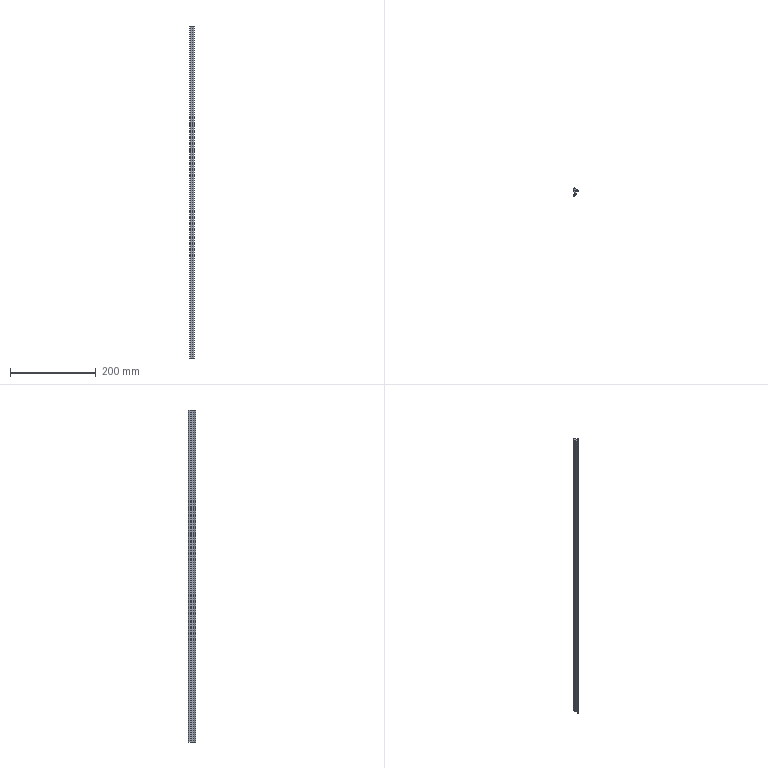Part | SolidWorks | features BaseBody 1, MoveFace 1 | 1 solid | 20 faces | box 10.8 x 17.5 x 774 mm | volume 60992 mm3 | cylinder 11 | plane 9 | commonest cylinder face diameters 1.6 x2 14 x2 0.4 x1 0.6 x1 0.8 x1 2.6 x1
STEP:
#1=CARTESIAN_POINT('',(-3.236,-11.055,674.));
#2=VERTEX_POINT('',#1);
#3=CARTESIAN_POINT('',(-4.3,-10.3,674.));
#4=VERTEX_POINT('',#3);
#5=CARTESIAN_POINT('',(-3.5,-10.3,674.));
#6=DIRECTION('',(0.,0.,-1.));
#7=DIRECTION('',(1.,0.,0.));
#8=AXIS2_PLACEMENT_3D('',#5,#6,#7);
#9=CIRCLE('',#8,0.8);
#10=EDGE_CURVE('',#2,#4,#9,.T.);
#11=ORIENTED_EDGE('',*,*,#10,.T.);
#12=CARTESIAN_POINT('',(-4.3,-10.3,-100.));
#13=VERTEX_POINT('',#12);
#14=CARTESIAN_POINT('',(-4.3,-10.3,-100.));
#15=DIRECTION('',(0.,0.,-1.));
#16=VECTOR('',#15,1000.);
#17=LINE('',#14,#16);
#18=EDGE_CURVE('',#4,#13,#17,.T.);
#19=ORIENTED_EDGE('',*,*,#18,.T.);
#20=CARTESIAN_POINT('',(-3.236,-11.055,-100.));
#21=VERTEX_POINT('',#20);
#22=CARTESIAN_POINT('',(-3.5,-10.3,-100.));
#23=DIRECTION('',(0.,0.,1.));
#24=DIRECTION('',(-1.,0.,0.));
#25=AXIS2_PLACEMENT_3D('',#22,#23,#24);
#26=CIRCLE('',#25,0.8);
#27=EDGE_CURVE('',#13,#21,#26,.T.);
#28=ORIENTED_EDGE('',*,*,#27,.T.);
#29=CARTESIAN_POINT('',(-3.236,-11.055,-100.));
#30=DIRECTION('',(0.,0.,-1.));
#31=VECTOR('',#30,1000.);
#32=LINE('',#29,#31);
#33=EDGE_CURVE('',#2,#21,#32,.T.);
#34=ORIENTED_EDGE('',*,*,#33,.F.);
#35=EDGE_LOOP('',(#11,#19,#28,#34));
#36=FACE_OUTER_BOUND('',#35,.T.);
#37=CARTESIAN_POINT('',(-3.5,-10.3,-100.));
#38=DIRECTION('',(0.,0.,-1.));
#39=DIRECTION('',(-1.,0.,0.));
#40=AXIS2_PLACEMENT_3D('',#37,#38,#39);
#41=CYLINDRICAL_SURFACE('',#40,0.8);
#42=ADVANCED_FACE('',(#36),#41,.T.);
#43=CARTESIAN_POINT('',(1.184,-6.397,-100.));
#44=VERTEX_POINT('',#43);
#45=CARTESIAN_POINT('',(-5.702,-4.29,-100.));
#46=DIRECTION('',(0.,0.,1.));
#47=DIRECTION('',(-1.,0.,0.));
#48=AXIS2_PLACEMENT_3D('',#45,#46,#47);
#49=CIRCLE('',#48,7.201);
#50=EDGE_CURVE('',#21,#44,#49,.T.);
#51=ORIENTED_EDGE('',*,*,#50,.T.);
#52=CARTESIAN_POINT('',(1.184,-6.397,674.));
#53=VERTEX_POINT('',#52);
#54=CARTESIAN_POINT('',(1.184,-6.397,-100.));
#55=DIRECTION('',(0.,0.,1.));
#56=VECTOR('',#55,1000.);
#57=LINE('',#54,#56);
#58=EDGE_CURVE('',#44,#53,#57,.T.);
#59=ORIENTED_EDGE('',*,*,#58,.T.);
#60=CARTESIAN_POINT('',(-5.702,-4.29,674.));
#61=DIRECTION('',(0.,0.,-1.));
#62=DIRECTION('',(1.,0.,0.));
#63=AXIS2_PLACEMENT_3D('',#60,#61,#62);
#64=CIRCLE('',#63,7.201);
#65=EDGE_CURVE('',#53,#2,#64,.T.);
#66=ORIENTED_EDGE('',*,*,#65,.T.);
#67=ORIENTED_EDGE('',*,*,#33,.T.);
#68=EDGE_LOOP('',(#51,#59,#66,#67));
#69=FACE_OUTER_BOUND('',#68,.T.);
#70=CARTESIAN_POINT('',(-5.702,-4.29,-100.));
#71=DIRECTION('',(0.,0.,-1.));
#72=DIRECTION('',(-1.,0.,0.));
#73=AXIS2_PLACEMENT_3D('',#70,#71,#72);
#74=CYLINDRICAL_SURFACE('',#73,7.201);
#75=ADVANCED_FACE('',(#69),#74,.T.);
#76=CARTESIAN_POINT('',(0.9,-6.,-100.));
#77=VERTEX_POINT('',#76);
#78=CARTESIAN_POINT('',(0.9,-6.3,-100.));
#79=DIRECTION('',(0.,0.,1.));
#80=DIRECTION('',(-1.,0.,0.));
#81=AXIS2_PLACEMENT_3D('',#78,#79,#80);
#82=CIRCLE('',#81,0.3);
#83=EDGE_CURVE('',#44,#77,#82,.T.);
#84=ORIENTED_EDGE('',*,*,#83,.T.);
#85=CARTESIAN_POINT('',(0.9,-6.,674.));
#86=VERTEX_POINT('',#85);
#87=CARTESIAN_POINT('',(0.9,-6.,-100.));
#88=DIRECTION('',(0.,0.,1.));
#89=VECTOR('',#88,1000.);
#90=LINE('',#87,#89);
#91=EDGE_CURVE('',#77,#86,#90,.T.);
#92=ORIENTED_EDGE('',*,*,#91,.T.);
#93=CARTESIAN_POINT('',(0.9,-6.3,674.));
#94=DIRECTION('',(0.,0.,-1.));
#95=DIRECTION('',(1.,0.,0.));
#96=AXIS2_PLACEMENT_3D('',#93,#94,#95);
#97=CIRCLE('',#96,0.3);
#98=EDGE_CURVE('',#86,#53,#97,.T.);
#99=ORIENTED_EDGE('',*,*,#98,.T.);
#100=ORIENTED_EDGE('',*,*,#58,.F.);
#101=EDGE_LOOP('',(#84,#92,#99,#100));
#102=FACE_OUTER_BOUND('',#101,.T.);
#103=CARTESIAN_POINT('',(0.9,-6.3,-100.));
#104=DIRECTION('',(0.,0.,-1.));
#105=DIRECTION('',(-1.,0.,0.));
#106=AXIS2_PLACEMENT_3D('',#103,#104,#105);
#107=CYLINDRICAL_SURFACE('',#106,0.3);
#108=ADVANCED_FACE('',(#102),#107,.T.);
#109=CARTESIAN_POINT('',(-2.5,-0.5,-100.));
#110=VERTEX_POINT('',#109);
#111=CARTESIAN_POINT('',(-2.5,-6.153,-100.));
#112=VERTEX_POINT('',#111);
#113=CARTESIAN_POINT('',(-2.5,-6.397,-100.));
#114=DIRECTION('',(0.,-1.,0.));
#115=VECTOR('',#114,1000.);
#116=LINE('',#113,#115);
#117=EDGE_CURVE('',#110,#112,#116,.T.);
#118=ORIENTED_EDGE('',*,*,#117,.F.);
#119=CARTESIAN_POINT('',(-4.2,1.695,-100.));
#120=VERTEX_POINT('',#119);
#121=CARTESIAN_POINT('',(-1.701,1.875,-100.));
#122=DIRECTION('',(0.,0.,1.));
#123=DIRECTION('',(-1.,0.,0.));
#124=AXIS2_PLACEMENT_3D('',#121,#122,#123);
#125=CIRCLE('',#124,2.506);
#126=EDGE_CURVE('',#120,#110,#125,.T.);
#127=ORIENTED_EDGE('',*,*,#126,.F.);
#128=CARTESIAN_POINT('',(-4.2,5.1,-100.));
#129=VERTEX_POINT('',#128);
#130=CARTESIAN_POINT('',(-4.2,-6.397,-100.));
#131=DIRECTION('',(0.,-1.,0.));
#132=VECTOR('',#131,1000.);
#133=LINE('',#130,#132);
#134=EDGE_CURVE('',#129,#120,#133,.T.);
#135=ORIENTED_EDGE('',*,*,#134,.F.);
#136=CARTESIAN_POINT('',(-2.892,6.4,-100.));
#137=VERTEX_POINT('',#136);
#138=CARTESIAN_POINT('',(-2.9,5.1,-100.));
#139=DIRECTION('',(0.,0.,1.));
#140=DIRECTION('',(-1.,0.,0.));
#141=AXIS2_PLACEMENT_3D('',#138,#139,#140);
#142=CIRCLE('',#141,1.3);
#143=EDGE_CURVE('',#137,#129,#142,.T.);
#144=ORIENTED_EDGE('',*,*,#143,.F.);
#145=CARTESIAN_POINT('',(0.5,5.5,-100.));
#146=VERTEX_POINT('',#145);
#147=CARTESIAN_POINT('',(-2.934,-0.5999,-100.));
#148=DIRECTION('',(0.,0.,1.));
#149=DIRECTION('',(-1.,0.,0.));
#150=AXIS2_PLACEMENT_3D('',#147,#148,#149);
#151=CIRCLE('',#150,7.);
#152=EDGE_CURVE('',#146,#137,#151,.T.);
#153=ORIENTED_EDGE('',*,*,#152,.F.);
#154=CARTESIAN_POINT('',(5.5,1.7,-100.));
#155=VERTEX_POINT('',#154);
#156=CARTESIAN_POINT('',(5.5,1.7,-100.));
#157=DIRECTION('',(-0.7962,0.6051,0.));
#158=VECTOR('',#157,1000.);
#159=LINE('',#156,#158);
#160=EDGE_CURVE('',#155,#146,#159,.T.);
#161=ORIENTED_EDGE('',*,*,#160,.F.);
#162=CARTESIAN_POINT('',(6.458,-0.2215,-100.));
#163=VERTEX_POINT('',#162);
#164=CARTESIAN_POINT('',(6.458,-0.2215,-100.));
#165=DIRECTION('',(-0.4462,0.8949,0.));
#166=VECTOR('',#165,1000.);
#167=LINE('',#164,#166);
#168=EDGE_CURVE('',#163,#155,#167,.T.);
#169=ORIENTED_EDGE('',*,*,#168,.F.);
#170=CARTESIAN_POINT('',(5.895,-0.7433,-100.));
#171=VERTEX_POINT('',#170);
#172=CARTESIAN_POINT('',(6.1,-0.4,-100.));
#173=DIRECTION('',(0.,0.,1.));
#174=DIRECTION('',(-1.,0.,0.));
#175=AXIS2_PLACEMENT_3D('',#172,#173,#174);
#176=CIRCLE('',#175,0.4);
#177=EDGE_CURVE('',#171,#163,#176,.T.);
#178=ORIENTED_EDGE('',*,*,#177,.F.);
#179=CARTESIAN_POINT('',(3.,0.,-100.));
#180=VERTEX_POINT('',#179);
#181=CARTESIAN_POINT('',(2.746,-6.995,-100.));
#182=DIRECTION('',(0.,0.,-1.));
#183=DIRECTION('',(-1.,0.,0.));
#184=AXIS2_PLACEMENT_3D('',#181,#182,#183);
#185=CIRCLE('',#184,7.);
#186=EDGE_CURVE('',#180,#171,#185,.T.);
#187=ORIENTED_EDGE('',*,*,#186,.F.);
#188=CARTESIAN_POINT('',(0.,0.,-100.));
#189=VERTEX_POINT('',#188);
#190=CARTESIAN_POINT('',(-6.814,0.,-100.));
#191=DIRECTION('',(1.,0.,0.));
#192=VECTOR('',#191,1000.);
#193=LINE('',#190,#192);
#194=EDGE_CURVE('',#189,#180,#193,.T.);
#195=ORIENTED_EDGE('',*,*,#194,.F.);
#196=CARTESIAN_POINT('',(0.,-5.8,-100.));
#197=VERTEX_POINT('',#196);
#198=CARTESIAN_POINT('',(0.,-6.397,-100.));
#199=DIRECTION('',(0.,1.,0.));
#200=VECTOR('',#199,1000.);
#201=LINE('',#198,#200);
#202=EDGE_CURVE('',#197,#189,#201,.T.);
#203=ORIENTED_EDGE('',*,*,#202,.F.);
#204=CARTESIAN_POINT('',(0.2,-6.,-100.));
#205=VERTEX_POINT('',#204);
#206=CARTESIAN_POINT('',(0.2,-5.8,-100.));
#207=DIRECTION('',(0.,0.,1.));
#208=DIRECTION('',(-1.,0.,0.));
#209=AXIS2_PLACEMENT_3D('',#206,#207,#208);
#210=CIRCLE('',#209,0.2);
#211=EDGE_CURVE('',#197,#205,#210,.T.);
#212=ORIENTED_EDGE('',*,*,#211,.T.);
#213=CARTESIAN_POINT('',(-6.814,-6.,-100.));
#214=DIRECTION('',(-1.,0.,0.));
#215=VECTOR('',#214,1000.);
#216=LINE('',#213,#215);
#217=EDGE_CURVE('',#77,#205,#216,.T.);
#218=ORIENTED_EDGE('',*,*,#217,.F.);
#219=ORIENTED_EDGE('',*,*,#83,.F.);
#220=ORIENTED_EDGE('',*,*,#50,.F.);
#221=ORIENTED_EDGE('',*,*,#27,.F.);
#222=CARTESIAN_POINT('',(-3.998,-9.674,-100.));
#223=VERTEX_POINT('',#222);
#224=CARTESIAN_POINT('',(-3.5,-10.3,-100.));
#225=DIRECTION('',(0.,0.,1.));
#226=DIRECTION('',(-1.,0.,0.));
#227=AXIS2_PLACEMENT_3D('',#224,#225,#226);
#228=CIRCLE('',#227,0.8);
#229=EDGE_CURVE('',#223,#13,#228,.T.);
#230=ORIENTED_EDGE('',*,*,#229,.F.);
#231=CARTESIAN_POINT('',(-6.814,-6.397,-100.));
#232=DIRECTION('',(0.,0.,-1.));
#233=DIRECTION('',(-1.,0.,0.));
#234=AXIS2_PLACEMENT_3D('',#231,#232,#233);
#235=CIRCLE('',#234,4.321);
#236=EDGE_CURVE('',#112,#223,#235,.T.);
#237=ORIENTED_EDGE('',*,*,#236,.F.);
#238=EDGE_LOOP('',(#118,#127,#135,#144,#153,#161,#169,#178,#187,#195,#203,#212,#218,#219,#220,#221,#230,#237));
#239=FACE_OUTER_BOUND('',#238,.T.);
#240=CARTESIAN_POINT('',(-6.814,-6.397,-100.));
#241=DIRECTION('',(0.,0.,1.));
#242=DIRECTION('',(1.,0.,0.));
#243=AXIS2_PLACEMENT_3D('',#240,#241,#242);
#244=PLANE('',#243);
#245=ADVANCED_FACE('',(#239),#244,.F.);
#246=ORIENTED_EDGE('',*,*,#18,.F.);
#247=CARTESIAN_POINT('',(-3.998,-9.674,674.));
#248=VERTEX_POINT('',#247);
#249=CARTESIAN_POINT('',(-3.5,-10.3,674.));
#250=DIRECTION('',(0.,0.,-1.));
#251=DIRECTION('',(1.,0.,0.));
#252=AXIS2_PLACEMENT_3D('',#249,#250,#251);
#253=CIRCLE('',#252,0.8);
#254=EDGE_CURVE('',#4,#248,#253,.T.);
#255=ORIENTED_EDGE('',*,*,#254,.T.);
#256=CARTESIAN_POINT('',(-3.998,-9.674,-100.));
#257=DIRECTION('',(0.,0.,-1.));
#258=VECTOR('',#257,1000.);
#259=LINE('',#256,#258);
#260=EDGE_CURVE('',#248,#223,#259,.T.);
#261=ORIENTED_EDGE('',*,*,#260,.T.);
#262=ORIENTED_EDGE('',*,*,#229,.T.);
#263=EDGE_LOOP('',(#246,#255,#261,#262));
#264=FACE_OUTER_BOUND('',#263,.T.);
#265=CARTESIAN_POINT('',(-3.5,-10.3,-100.));
#266=DIRECTION('',(0.,0.,-1.));
#267=DIRECTION('',(-1.,0.,0.));
#268=AXIS2_PLACEMENT_3D('',#265,#266,#267);
#269=CYLINDRICAL_SURFACE('',#268,0.8);
#270=ADVANCED_FACE('',(#264),#269,.T.);
#271=CARTESIAN_POINT('',(-4.2,1.695,674.));
#272=VERTEX_POINT('',#271);
#273=CARTESIAN_POINT('',(-2.5,-0.5,674.));
#274=VERTEX_POINT('',#273);
#275=CARTESIAN_POINT('',(-1.701,1.875,674.));
#276=DIRECTION('',(0.,0.,1.));
#277=DIRECTION('',(1.,0.,0.));
#278=AXIS2_PLACEMENT_3D('',#275,#276,#277);
#279=CIRCLE('',#278,2.506);
#280=EDGE_CURVE('',#272,#274,#279,.T.);
#281=ORIENTED_EDGE('',*,*,#280,.T.);
#282=CARTESIAN_POINT('',(-2.5,-6.153,674.));
#283=VERTEX_POINT('',#282);
#284=CARTESIAN_POINT('',(-2.5,-6.397,674.));
#285=DIRECTION('',(0.,-1.,0.));
#286=VECTOR('',#285,1000.);
#287=LINE('',#284,#286);
#288=EDGE_CURVE('',#274,#283,#287,.T.);
#289=ORIENTED_EDGE('',*,*,#288,.T.);
#290=CARTESIAN_POINT('',(-6.814,-6.397,674.));
#291=DIRECTION('',(0.,0.,-1.));
#292=DIRECTION('',(1.,0.,0.));
#293=AXIS2_PLACEMENT_3D('',#290,#291,#292);
#294=CIRCLE('',#293,4.321);
#295=EDGE_CURVE('',#283,#248,#294,.T.);
#296=ORIENTED_EDGE('',*,*,#295,.T.);
#297=ORIENTED_EDGE('',*,*,#254,.F.);
#298=ORIENTED_EDGE('',*,*,#10,.F.);
#299=ORIENTED_EDGE('',*,*,#65,.F.);
#300=ORIENTED_EDGE('',*,*,#98,.F.);
#301=CARTESIAN_POINT('',(0.2,-6.,674.));
#302=VERTEX_POINT('',#301);
#303=CARTESIAN_POINT('',(-6.814,-6.,674.));
#304=DIRECTION('',(-1.,0.,0.));
#305=VECTOR('',#304,1000.);
#306=LINE('',#303,#305);
#307=EDGE_CURVE('',#86,#302,#306,.T.);
#308=ORIENTED_EDGE('',*,*,#307,.T.);
#309=CARTESIAN_POINT('',(0.,-5.8,674.));
#310=VERTEX_POINT('',#309);
#311=CARTESIAN_POINT('',(0.2,-5.8,674.));
#312=DIRECTION('',(0.,0.,-1.));
#313=DIRECTION('',(1.,0.,0.));
#314=AXIS2_PLACEMENT_3D('',#311,#312,#313);
#315=CIRCLE('',#314,0.2);
#316=EDGE_CURVE('',#302,#310,#315,.T.);
#317=ORIENTED_EDGE('',*,*,#316,.T.);
#318=CARTESIAN_POINT('',(0.,0.,674.));
#319=VERTEX_POINT('',#318);
#320=CARTESIAN_POINT('',(0.,-6.397,674.));
#321=DIRECTION('',(0.,1.,0.));
#322=VECTOR('',#321,1000.);
#323=LINE('',#320,#322);
#324=EDGE_CURVE('',#310,#319,#323,.T.);
#325=ORIENTED_EDGE('',*,*,#324,.T.);
#326=CARTESIAN_POINT('',(3.,0.,674.));
#327=VERTEX_POINT('',#326);
#328=CARTESIAN_POINT('',(-6.814,0.,674.));
#329=DIRECTION('',(1.,0.,0.));
#330=VECTOR('',#329,1000.);
#331=LINE('',#328,#330);
#332=EDGE_CURVE('',#319,#327,#331,.T.);
#333=ORIENTED_EDGE('',*,*,#332,.T.);
#334=CARTESIAN_POINT('',(5.895,-0.7433,674.));
#335=VERTEX_POINT('',#334);
#336=CARTESIAN_POINT('',(2.746,-6.995,674.));
#337=DIRECTION('',(0.,0.,-1.));
#338=DIRECTION('',(1.,0.,0.));
#339=AXIS2_PLACEMENT_3D('',#336,#337,#338);
#340=CIRCLE('',#339,7.);
#341=EDGE_CURVE('',#327,#335,#340,.T.);
#342=ORIENTED_EDGE('',*,*,#341,.T.);
#343=CARTESIAN_POINT('',(6.458,-0.2215,674.));
#344=VERTEX_POINT('',#343);
#345=CARTESIAN_POINT('',(6.1,-0.4,674.));
#346=DIRECTION('',(0.,0.,-1.));
#347=DIRECTION('',(1.,0.,0.));
#348=AXIS2_PLACEMENT_3D('',#345,#346,#347);
#349=CIRCLE('',#348,0.4);
#350=EDGE_CURVE('',#344,#335,#349,.T.);
#351=ORIENTED_EDGE('',*,*,#350,.F.);
#352=CARTESIAN_POINT('',(5.5,1.7,674.));
#353=VERTEX_POINT('',#352);
#354=CARTESIAN_POINT('',(6.282,0.1323,674.));
#355=DIRECTION('',(-0.4462,0.8949,0.));
#356=VECTOR('',#355,1000.);
#357=LINE('',#354,#356);
#358=EDGE_CURVE('',#344,#353,#357,.T.);
#359=ORIENTED_EDGE('',*,*,#358,.T.);
#360=CARTESIAN_POINT('',(0.5,5.5,674.));
#361=VERTEX_POINT('',#360);
#362=CARTESIAN_POINT('',(1.595,4.668,674.));
#363=DIRECTION('',(-0.7962,0.6051,0.));
#364=VECTOR('',#363,1000.);
#365=LINE('',#362,#364);
#366=EDGE_CURVE('',#353,#361,#365,.T.);
#367=ORIENTED_EDGE('',*,*,#366,.T.);
#368=CARTESIAN_POINT('',(-2.892,6.4,674.));
#369=VERTEX_POINT('',#368);
#370=CARTESIAN_POINT('',(-2.934,-0.5999,674.));
#371=DIRECTION('',(0.,0.,1.));
#372=DIRECTION('',(1.,0.,0.));
#373=AXIS2_PLACEMENT_3D('',#370,#371,#372);
#374=CIRCLE('',#373,7.);
#375=EDGE_CURVE('',#361,#369,#374,.T.);
#376=ORIENTED_EDGE('',*,*,#375,.T.);
#377=CARTESIAN_POINT('',(-4.2,5.1,674.));
#378=VERTEX_POINT('',#377);
#379=CARTESIAN_POINT('',(-2.9,5.1,674.));
#380=DIRECTION('',(0.,0.,1.));
#381=DIRECTION('',(1.,0.,0.));
#382=AXIS2_PLACEMENT_3D('',#379,#380,#381);
#383=CIRCLE('',#382,1.3);
#384=EDGE_CURVE('',#369,#378,#383,.T.);
#385=ORIENTED_EDGE('',*,*,#384,.T.);
#386=CARTESIAN_POINT('',(-4.2,-6.397,674.));
#387=DIRECTION('',(0.,-1.,0.));
#388=VECTOR('',#387,1000.);
#389=LINE('',#386,#388);
#390=EDGE_CURVE('',#378,#272,#389,.T.);
#391=ORIENTED_EDGE('',*,*,#390,.T.);
#392=EDGE_LOOP('',(#281,#289,#296,#297,#298,#299,#300,#308,#317,#325,#333,#342,#351,#359,#367,#376,#385,#391));
#393=FACE_OUTER_BOUND('',#392,.T.);
#394=CARTESIAN_POINT('',(-6.814,-6.397,674.));
#395=DIRECTION('',(0.,0.,1.));
#396=DIRECTION('',(1.,0.,0.));
#397=AXIS2_PLACEMENT_3D('',#394,#395,#396);
#398=PLANE('',#397);
#399=ADVANCED_FACE('',(#393),#398,.T.);
#400=ORIENTED_EDGE('',*,*,#217,.T.);
#401=CARTESIAN_POINT('',(0.2,-6.,-100.));
#402=DIRECTION('',(0.,0.,1.));
#403=VECTOR('',#402,1000.);
#404=LINE('',#401,#403);
#405=EDGE_CURVE('',#205,#302,#404,.T.);
#406=ORIENTED_EDGE('',*,*,#405,.T.);
#407=ORIENTED_EDGE('',*,*,#307,.F.);
#408=ORIENTED_EDGE('',*,*,#91,.F.);
#409=EDGE_LOOP('',(#400,#406,#407,#408));
#410=FACE_OUTER_BOUND('',#409,.T.);
#411=CARTESIAN_POINT('',(0.9,-6.,-100.));
#412=DIRECTION('',(0.,1.,0.));
#413=DIRECTION('',(0.,0.,1.));
#414=AXIS2_PLACEMENT_3D('',#411,#412,#413);
#415=PLANE('',#414);
#416=ADVANCED_FACE('',(#410),#415,.T.);
#417=CARTESIAN_POINT('',(-2.5,-6.153,-100.));
#418=DIRECTION('',(0.,0.,1.));
#419=VECTOR('',#418,1000.);
#420=LINE('',#417,#419);
#421=EDGE_CURVE('',#112,#283,#420,.T.);
#422=ORIENTED_EDGE('',*,*,#421,.F.);
#423=ORIENTED_EDGE('',*,*,#236,.T.);
#424=ORIENTED_EDGE('',*,*,#260,.F.);
#425=ORIENTED_EDGE('',*,*,#295,.F.);
#426=EDGE_LOOP('',(#422,#423,#424,#425));
#427=FACE_OUTER_BOUND('',#426,.T.);
#428=CARTESIAN_POINT('',(-6.814,-6.397,-100.));
#429=DIRECTION('',(0.,0.,-1.));
#430=DIRECTION('',(-1.,0.,0.));
#431=AXIS2_PLACEMENT_3D('',#428,#429,#430);
#432=CYLINDRICAL_SURFACE('',#431,4.321);
#433=ADVANCED_FACE('',(#427),#432,.F.);
#434=ORIENTED_EDGE('',*,*,#117,.T.);
#435=ORIENTED_EDGE('',*,*,#421,.T.);
#436=ORIENTED_EDGE('',*,*,#288,.F.);
#437=CARTESIAN_POINT('',(-2.5,-0.5,-100.));
#438=DIRECTION('',(0.,0.,-1.));
#439=VECTOR('',#438,1000.);
#440=LINE('',#437,#439);
#441=EDGE_CURVE('',#274,#110,#440,.T.);
#442=ORIENTED_EDGE('',*,*,#441,.T.);
#443=EDGE_LOOP('',(#434,#435,#436,#442));
#444=FACE_OUTER_BOUND('',#443,.T.);
#445=CARTESIAN_POINT('',(-2.5,-0.5,-100.));
#446=DIRECTION('',(-1.,0.,0.));
#447=DIRECTION('',(0.,0.,1.));
#448=AXIS2_PLACEMENT_3D('',#445,#446,#447);
#449=PLANE('',#448);
#450=ADVANCED_FACE('',(#444),#449,.T.);
#451=ORIENTED_EDGE('',*,*,#126,.T.);
#452=ORIENTED_EDGE('',*,*,#441,.F.);
#453=ORIENTED_EDGE('',*,*,#280,.F.);
#454=CARTESIAN_POINT('',(-4.2,1.695,-100.));
#455=DIRECTION('',(0.,0.,-1.));
#456=VECTOR('',#455,1000.);
#457=LINE('',#454,#456);
#458=EDGE_CURVE('',#272,#120,#457,.T.);
#459=ORIENTED_EDGE('',*,*,#458,.T.);
#460=EDGE_LOOP('',(#451,#452,#453,#459));
#461=FACE_OUTER_BOUND('',#460,.T.);
#462=CARTESIAN_POINT('',(-1.701,1.875,-100.));
#463=DIRECTION('',(0.,0.,-1.));
#464=DIRECTION('',(-1.,0.,0.));
#465=AXIS2_PLACEMENT_3D('',#462,#463,#464);
#466=CYLINDRICAL_SURFACE('',#465,2.506);
#467=ADVANCED_FACE('',(#461),#466,.T.);
#468=ORIENTED_EDGE('',*,*,#134,.T.);
#469=ORIENTED_EDGE('',*,*,#458,.F.);
#470=ORIENTED_EDGE('',*,*,#390,.F.);
#471=CARTESIAN_POINT('',(-4.2,5.1,-100.));
#472=DIRECTION('',(0.,0.,-1.));
#473=VECTOR('',#472,1000.);
#474=LINE('',#471,#473);
#475=EDGE_CURVE('',#378,#129,#474,.T.);
#476=ORIENTED_EDGE('',*,*,#475,.T.);
#477=EDGE_LOOP('',(#468,#469,#470,#476));
#478=FACE_OUTER_BOUND('',#477,.T.);
#479=CARTESIAN_POINT('',(-4.2,5.1,-100.));
#480=DIRECTION('',(-1.,0.,0.));
#481=DIRECTION('',(0.,0.,1.));
#482=AXIS2_PLACEMENT_3D('',#479,#480,#481);
#483=PLANE('',#482);
#484=ADVANCED_FACE('',(#478),#483,.T.);
#485=ORIENTED_EDGE('',*,*,#143,.T.);
#486=ORIENTED_EDGE('',*,*,#475,.F.);
#487=ORIENTED_EDGE('',*,*,#384,.F.);
#488=CARTESIAN_POINT('',(-2.892,6.4,-100.));
#489=DIRECTION('',(0.,0.,-1.));
#490=VECTOR('',#489,1000.);
#491=LINE('',#488,#490);
#492=EDGE_CURVE('',#369,#137,#491,.T.);
#493=ORIENTED_EDGE('',*,*,#492,.T.);
#494=EDGE_LOOP('',(#485,#486,#487,#493));
#495=FACE_OUTER_BOUND('',#494,.T.);
#496=CARTESIAN_POINT('',(-2.9,5.1,-100.));
#497=DIRECTION('',(0.,0.,-1.));
#498=DIRECTION('',(-1.,0.,0.));
#499=AXIS2_PLACEMENT_3D('',#496,#497,#498);
#500=CYLINDRICAL_SURFACE('',#499,1.3);
#501=ADVANCED_FACE('',(#495),#500,.T.);
#502=ORIENTED_EDGE('',*,*,#152,.T.);
#503=ORIENTED_EDGE('',*,*,#492,.F.);
#504=ORIENTED_EDGE('',*,*,#375,.F.);
#505=CARTESIAN_POINT('',(0.5,5.5,-100.));
#506=DIRECTION('',(0.,0.,-1.));
#507=VECTOR('',#506,1000.);
#508=LINE('',#505,#507);
#509=EDGE_CURVE('',#361,#146,#508,.T.);
#510=ORIENTED_EDGE('',*,*,#509,.T.);
#511=EDGE_LOOP('',(#502,#503,#504,#510));
#512=FACE_OUTER_BOUND('',#511,.T.);
#513=CARTESIAN_POINT('',(-2.934,-0.5999,-100.));
#514=DIRECTION('',(0.,0.,-1.));
#515=DIRECTION('',(-1.,0.,0.));
#516=AXIS2_PLACEMENT_3D('',#513,#514,#515);
#517=CYLINDRICAL_SURFACE('',#516,7.);
#518=ADVANCED_FACE('',(#512),#517,.T.);
#519=ORIENTED_EDGE('',*,*,#160,.T.);
#520=ORIENTED_EDGE('',*,*,#509,.F.);
#521=ORIENTED_EDGE('',*,*,#366,.F.);
#522=CARTESIAN_POINT('',(5.5,1.7,-100.));
#523=DIRECTION('',(0.,0.,-1.));
#524=VECTOR('',#523,1000.);
#525=LINE('',#522,#524);
#526=EDGE_CURVE('',#353,#155,#525,.T.);
#527=ORIENTED_EDGE('',*,*,#526,.T.);
#528=EDGE_LOOP('',(#519,#520,#521,#527));
#529=FACE_OUTER_BOUND('',#528,.T.);
#530=CARTESIAN_POINT('',(5.5,1.7,-100.));
#531=DIRECTION('',(0.6051,0.7962,0.));
#532=DIRECTION('',(-0.7962,0.6051,0.));
#533=AXIS2_PLACEMENT_3D('',#530,#531,#532);
#534=PLANE('',#533);
#535=ADVANCED_FACE('',(#529),#534,.T.);
#536=ORIENTED_EDGE('',*,*,#168,.T.);
#537=ORIENTED_EDGE('',*,*,#526,.F.);
#538=ORIENTED_EDGE('',*,*,#358,.F.);
#539=CARTESIAN_POINT('',(6.458,-0.2215,-100.));
#540=DIRECTION('',(0.,0.,-1.));
#541=VECTOR('',#540,1000.);
#542=LINE('',#539,#541);
#543=EDGE_CURVE('',#344,#163,#542,.T.);
#544=ORIENTED_EDGE('',*,*,#543,.T.);
#545=EDGE_LOOP('',(#536,#537,#538,#544));
#546=FACE_OUTER_BOUND('',#545,.T.);
#547=CARTESIAN_POINT('',(6.458,-0.2215,-100.));
#548=DIRECTION('',(0.8949,0.4462,0.));
#549=DIRECTION('',(-0.4462,0.8949,0.));
#550=AXIS2_PLACEMENT_3D('',#547,#548,#549);
#551=PLANE('',#550);
#552=ADVANCED_FACE('',(#546),#551,.T.);
#553=CARTESIAN_POINT('',(3.,0.,-100.));
#554=DIRECTION('',(0.,0.,1.));
#555=VECTOR('',#554,1000.);
#556=LINE('',#553,#555);
#557=EDGE_CURVE('',#180,#327,#556,.T.);
#558=ORIENTED_EDGE('',*,*,#557,.F.);
#559=ORIENTED_EDGE('',*,*,#186,.T.);
#560=CARTESIAN_POINT('',(5.895,-0.7433,-100.));
#561=DIRECTION('',(0.,0.,-1.));
#562=VECTOR('',#561,1000.);
#563=LINE('',#560,#562);
#564=EDGE_CURVE('',#335,#171,#563,.T.);
#565=ORIENTED_EDGE('',*,*,#564,.F.);
#566=ORIENTED_EDGE('',*,*,#341,.F.);
#567=EDGE_LOOP('',(#558,#559,#565,#566));
#568=FACE_OUTER_BOUND('',#567,.T.);
#569=CARTESIAN_POINT('',(2.746,-6.995,-100.));
#570=DIRECTION('',(0.,0.,-1.));
#571=DIRECTION('',(-1.,0.,0.));
#572=AXIS2_PLACEMENT_3D('',#569,#570,#571);
#573=CYLINDRICAL_SURFACE('',#572,7.);
#574=ADVANCED_FACE('',(#568),#573,.F.);
#575=ORIENTED_EDGE('',*,*,#194,.T.);
#576=ORIENTED_EDGE('',*,*,#557,.T.);
#577=ORIENTED_EDGE('',*,*,#332,.F.);
#578=CARTESIAN_POINT('',(0.,0.,-100.));
#579=DIRECTION('',(0.,0.,-1.));
#580=VECTOR('',#579,1000.);
#581=LINE('',#578,#580);
#582=EDGE_CURVE('',#319,#189,#581,.T.);
#583=ORIENTED_EDGE('',*,*,#582,.T.);
#584=EDGE_LOOP('',(#575,#576,#577,#583));
#585=FACE_OUTER_BOUND('',#584,.T.);
#586=CARTESIAN_POINT('',(0.,0.,-100.));
#587=DIRECTION('',(0.,-1.,0.));
#588=DIRECTION('',(0.,0.,-1.));
#589=AXIS2_PLACEMENT_3D('',#586,#587,#588);
#590=PLANE('',#589);
#591=ADVANCED_FACE('',(#585),#590,.T.);
#592=ORIENTED_EDGE('',*,*,#202,.T.);
#593=ORIENTED_EDGE('',*,*,#582,.F.);
#594=ORIENTED_EDGE('',*,*,#324,.F.);
#595=CARTESIAN_POINT('',(0.,-5.8,-100.));
#596=DIRECTION('',(0.,0.,-1.));
#597=VECTOR('',#596,1000.);
#598=LINE('',#595,#597);
#599=EDGE_CURVE('',#310,#197,#598,.T.);
#600=ORIENTED_EDGE('',*,*,#599,.T.);
#601=EDGE_LOOP('',(#592,#593,#594,#600));
#602=FACE_OUTER_BOUND('',#601,.T.);
#603=CARTESIAN_POINT('',(0.,-5.8,-100.));
#604=DIRECTION('',(1.,0.,0.));
#605=DIRECTION('',(0.,0.,-1.));
#606=AXIS2_PLACEMENT_3D('',#603,#604,#605);
#607=PLANE('',#606);
#608=ADVANCED_FACE('',(#602),#607,.T.);
#609=ORIENTED_EDGE('',*,*,#405,.F.);
#610=ORIENTED_EDGE('',*,*,#211,.F.);
#611=ORIENTED_EDGE('',*,*,#599,.F.);
#612=ORIENTED_EDGE('',*,*,#316,.F.);
#613=EDGE_LOOP('',(#609,#610,#611,#612));
#614=FACE_OUTER_BOUND('',#613,.T.);
#615=CARTESIAN_POINT('',(0.2,-5.8,-100.));
#616=DIRECTION('',(0.,0.,-1.));
#617=DIRECTION('',(-1.,0.,0.));
#618=AXIS2_PLACEMENT_3D('',#615,#616,#617);
#619=CYLINDRICAL_SURFACE('',#618,0.2);
#620=ADVANCED_FACE('',(#614),#619,.F.);
#621=ORIENTED_EDGE('',*,*,#177,.T.);
#622=ORIENTED_EDGE('',*,*,#543,.F.);
#623=ORIENTED_EDGE('',*,*,#350,.T.);
#624=ORIENTED_EDGE('',*,*,#564,.T.);
#625=EDGE_LOOP('',(#621,#622,#623,#624));
#626=FACE_OUTER_BOUND('',#625,.T.);
#627=CARTESIAN_POINT('',(6.1,-0.4,-100.));
#628=DIRECTION('',(0.,0.,-1.));
#629=DIRECTION('',(-1.,0.,0.));
#630=AXIS2_PLACEMENT_3D('',#627,#628,#629);
#631=CYLINDRICAL_SURFACE('',#630,0.4);
#632=ADVANCED_FACE('',(#626),#631,.T.);
#633=CLOSED_SHELL('',(#42,#75,#108,#245,#270,#399,#416,#433,#450,#467,#484,#501,#518,#535,#552,#574,#591,#608,#620,#632));
#634=MANIFOLD_SOLID_BREP('',#633);
#635=CARTESIAN_POINT('',(0.,0.,0.));
#636=DIRECTION('',(0.,0.,1.));
#637=DIRECTION('',(1.,0.,0.));
#638=AXIS2_PLACEMENT_3D('',#635,#636,#637);
#639=(LENGTH_UNIT()NAMED_UNIT(*)SI_UNIT(.MILLI.,.METRE.));
#640=UNCERTAINTY_MEASURE_WITH_UNIT(LENGTH_MEASURE(0.00001),#639,'','');
#641=(NAMED_UNIT(*)PLANE_ANGLE_UNIT()SI_UNIT($,.RADIAN.));
#642=(NAMED_UNIT(*)SI_UNIT($,.STERADIAN.)SOLID_ANGLE_UNIT());
#643=(GEOMETRIC_REPRESENTATION_CONTEXT(3)GLOBAL_UNCERTAINTY_ASSIGNED_CONTEXT((#640))GLOBAL_UNIT_ASSIGNED_CONTEXT((#639,#641,#642))REPRESENTATION_CONTEXT('',''));
#644=ADVANCED_BREP_SHAPE_REPRESENTATION('',(#634,#638),#643);